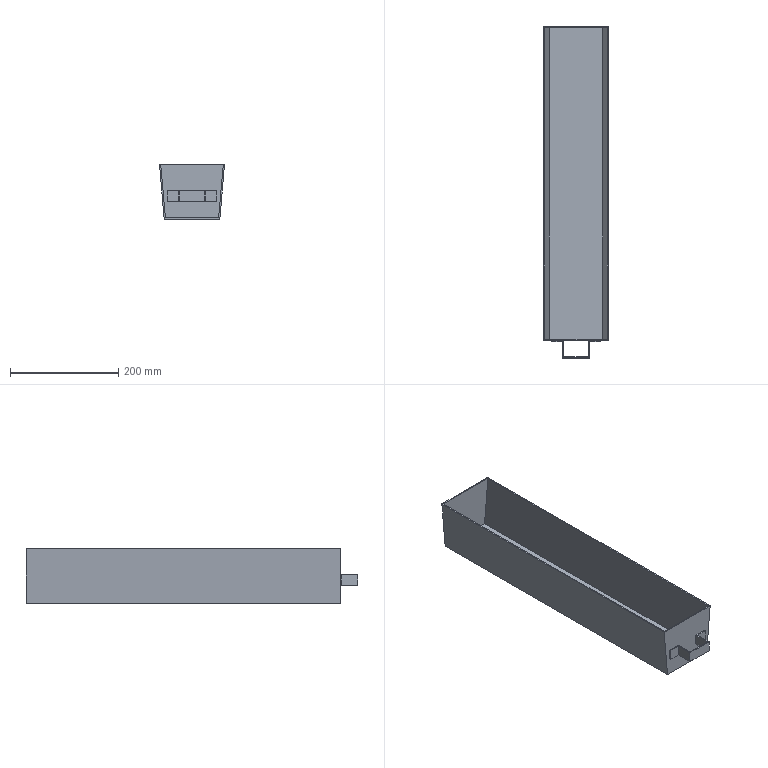Part | NX | features solid 2 | 1 solid | 23 faces | box 120 x 612.3 x 100 mm | volume 446880 mm3 | plane 19 | spline 4
STEP:
#1=CARTESIAN_POINT('',(80.865,-687.8,-515.5));
#2=VERTEX_POINT('',#1);
#3=CARTESIAN_POINT('',(179.135,-687.8,-515.5));
#4=VERTEX_POINT('',#3);
#5=CARTESIAN_POINT('',(-1370.,-687.8,-515.5));
#6=DIRECTION('',(-1.,0.,0.));
#7=VECTOR('',#6,1000.);
#8=LINE('',#5,#7);
#9=EDGE_CURVE('',#2,#4,#8,.F.);
#10=ORIENTED_EDGE('',*,*,#9,.T.);
#11=CARTESIAN_POINT('',(179.135,-112.3,-515.5));
#12=VERTEX_POINT('',#11);
#13=CARTESIAN_POINT('',(179.135,-112.3,-515.5));
#14=CARTESIAN_POINT('',(179.135,-304.133,-515.5));
#15=CARTESIAN_POINT('',(179.135,-495.967,-515.5));
#16=CARTESIAN_POINT('',(179.135,-687.8,-515.5));
#17=B_SPLINE_CURVE_WITH_KNOTS('',3,(#13,#14,#15,#16),.UNSPECIFIED.,.F.,.F.,(4,4),(0.,0.5755),.UNSPECIFIED.);
#18=EDGE_CURVE('',#12,#4,#17,.T.);
#19=ORIENTED_EDGE('',*,*,#18,.F.);
#20=CARTESIAN_POINT('',(80.865,-112.3,-515.5));
#21=VERTEX_POINT('',#20);
#22=CARTESIAN_POINT('',(896.442,-112.3,-515.5));
#23=DIRECTION('',(1.,0.,0.));
#24=VECTOR('',#23,1000.);
#25=LINE('',#22,#24);
#26=EDGE_CURVE('',#21,#12,#25,.T.);
#27=ORIENTED_EDGE('',*,*,#26,.F.);
#28=CARTESIAN_POINT('',(80.865,-687.8,-515.5));
#29=CARTESIAN_POINT('',(80.865,-495.967,-515.5));
#30=CARTESIAN_POINT('',(80.865,-304.133,-515.5));
#31=CARTESIAN_POINT('',(80.865,-112.3,-515.5));
#32=B_SPLINE_CURVE_WITH_KNOTS('',3,(#28,#29,#30,#31),.UNSPECIFIED.,.F.,.F.,(4,4),(0.,0.5755),.UNSPECIFIED.);
#33=EDGE_CURVE('',#2,#21,#32,.T.);
#34=ORIENTED_EDGE('',*,*,#33,.F.);
#35=EDGE_LOOP('',(#10,#19,#27,#34));
#36=FACE_BOUND('',#35,.T.);
#37=CARTESIAN_POINT('',(-1370.,-20.,-515.5));
#38=DIRECTION('',(0.,0.,-1.));
#39=DIRECTION('',(-1.,0.,0.));
#40=AXIS2_PLACEMENT_3D('',#37,#38,#39);
#41=PLANE('',#40);
#42=ADVANCED_FACE('',(#36),#41,.F.);
#43=CARTESIAN_POINT('',(187.691,-687.8,-417.7));
#44=VERTEX_POINT('',#43);
#45=CARTESIAN_POINT('',(187.691,-687.8,-417.7));
#46=CARTESIAN_POINT('',(184.839,-687.8,-450.3));
#47=CARTESIAN_POINT('',(181.987,-687.8,-482.9));
#48=CARTESIAN_POINT('',(179.135,-687.8,-515.5));
#49=B_SPLINE_CURVE_WITH_KNOTS('',3,(#45,#46,#47,#48),.UNSPECIFIED.,.F.,.F.,(4,4),(0.,0.09817),.UNSPECIFIED.);
#50=EDGE_CURVE('',#44,#4,#49,.T.);
#51=ORIENTED_EDGE('',*,*,#50,.F.);
#52=CARTESIAN_POINT('',(187.691,-112.3,-417.7));
#53=VERTEX_POINT('',#52);
#54=CARTESIAN_POINT('',(187.691,-112.3,-417.7));
#55=CARTESIAN_POINT('',(187.691,-304.133,-417.7));
#56=CARTESIAN_POINT('',(187.691,-495.967,-417.7));
#57=CARTESIAN_POINT('',(187.691,-687.8,-417.7));
#58=B_SPLINE_CURVE_WITH_KNOTS('',3,(#54,#55,#56,#57),.UNSPECIFIED.,.F.,.F.,(4,4),(0.,0.5755),.UNSPECIFIED.);
#59=EDGE_CURVE('',#53,#44,#58,.T.);
#60=ORIENTED_EDGE('',*,*,#59,.F.);
#61=CARTESIAN_POINT('',(187.691,-112.3,-417.7));
#62=CARTESIAN_POINT('',(184.839,-112.3,-450.3));
#63=CARTESIAN_POINT('',(181.987,-112.3,-482.9));
#64=CARTESIAN_POINT('',(179.135,-112.3,-515.5));
#65=B_SPLINE_CURVE_WITH_KNOTS('',3,(#61,#62,#63,#64),.UNSPECIFIED.,.F.,.F.,(4,4),(0.,0.09817),.UNSPECIFIED.);
#66=EDGE_CURVE('',#53,#12,#65,.T.);
#67=ORIENTED_EDGE('',*,*,#66,.T.);
#68=ORIENTED_EDGE('',*,*,#18,.T.);
#69=EDGE_LOOP('',(#51,#60,#67,#68));
#70=FACE_BOUND('',#69,.T.);
#71=CARTESIAN_POINT('',(179.135,-687.8,-515.5));
#72=CARTESIAN_POINT('',(179.135,-495.967,-515.5));
#73=CARTESIAN_POINT('',(179.135,-304.133,-515.5));
#74=CARTESIAN_POINT('',(179.135,-112.3,-515.5));
#75=CARTESIAN_POINT('',(181.987,-687.8,-482.9));
#76=CARTESIAN_POINT('',(181.987,-495.967,-482.9));
#77=CARTESIAN_POINT('',(181.987,-304.133,-482.9));
#78=CARTESIAN_POINT('',(181.987,-112.3,-482.9));
#79=CARTESIAN_POINT('',(184.839,-687.8,-450.3));
#80=CARTESIAN_POINT('',(184.839,-495.967,-450.3));
#81=CARTESIAN_POINT('',(184.839,-304.133,-450.3));
#82=CARTESIAN_POINT('',(184.839,-112.3,-450.3));
#83=CARTESIAN_POINT('',(187.691,-687.8,-417.7));
#84=CARTESIAN_POINT('',(187.691,-495.967,-417.7));
#85=CARTESIAN_POINT('',(187.691,-304.133,-417.7));
#86=CARTESIAN_POINT('',(187.691,-112.3,-417.7));
#87=B_SPLINE_SURFACE_WITH_KNOTS('',3,3,((#71,#72,#73,#74),(#75,#76,#77,#78),(#79,#80,#81,#82),(#83,#84,#85,#86)),.UNSPECIFIED.,.F.,.F.,.F.,(4,4),(4,4),(0.01625,0.998),(0.003793,0.996),.UNSPECIFIED.);
#88=ADVANCED_FACE('',(#70),#87,.T.);
#89=ORIENTED_EDGE('',*,*,#33,.T.);
#90=CARTESIAN_POINT('',(72.309,-112.3,-417.7));
#91=VERTEX_POINT('',#90);
#92=CARTESIAN_POINT('',(80.865,-112.3,-515.5));
#93=CARTESIAN_POINT('',(78.013,-112.3,-482.9));
#94=CARTESIAN_POINT('',(75.161,-112.3,-450.3));
#95=CARTESIAN_POINT('',(72.309,-112.3,-417.7));
#96=B_SPLINE_CURVE_WITH_KNOTS('',3,(#92,#93,#94,#95),.UNSPECIFIED.,.F.,.F.,(4,4),(0.,0.09817),.UNSPECIFIED.);
#97=EDGE_CURVE('',#21,#91,#96,.T.);
#98=ORIENTED_EDGE('',*,*,#97,.T.);
#99=CARTESIAN_POINT('',(72.309,-687.8,-417.7));
#100=VERTEX_POINT('',#99);
#101=CARTESIAN_POINT('',(72.309,-112.3,-417.7));
#102=CARTESIAN_POINT('',(72.309,-304.133,-417.7));
#103=CARTESIAN_POINT('',(72.309,-495.967,-417.7));
#104=CARTESIAN_POINT('',(72.309,-687.8,-417.7));
#105=B_SPLINE_CURVE_WITH_KNOTS('',3,(#101,#102,#103,#104),.UNSPECIFIED.,.F.,.F.,(4,4),(0.,0.5755),.UNSPECIFIED.);
#106=EDGE_CURVE('',#91,#100,#105,.T.);
#107=ORIENTED_EDGE('',*,*,#106,.T.);
#108=CARTESIAN_POINT('',(80.865,-687.8,-515.5));
#109=CARTESIAN_POINT('',(78.013,-687.8,-482.9));
#110=CARTESIAN_POINT('',(75.161,-687.8,-450.3));
#111=CARTESIAN_POINT('',(72.309,-687.8,-417.7));
#112=B_SPLINE_CURVE_WITH_KNOTS('',3,(#108,#109,#110,#111),.UNSPECIFIED.,.F.,.F.,(4,4),(0.,0.09817),.UNSPECIFIED.);
#113=EDGE_CURVE('',#2,#100,#112,.T.);
#114=ORIENTED_EDGE('',*,*,#113,.F.);
#115=EDGE_LOOP('',(#89,#98,#107,#114));
#116=FACE_BOUND('',#115,.T.);
#117=CARTESIAN_POINT('',(80.865,-687.8,-515.5));
#118=CARTESIAN_POINT('',(80.865,-495.967,-515.5));
#119=CARTESIAN_POINT('',(80.865,-304.133,-515.5));
#120=CARTESIAN_POINT('',(80.865,-112.3,-515.5));
#121=CARTESIAN_POINT('',(78.013,-687.8,-482.9));
#122=CARTESIAN_POINT('',(78.013,-495.967,-482.9));
#123=CARTESIAN_POINT('',(78.013,-304.133,-482.9));
#124=CARTESIAN_POINT('',(78.013,-112.3,-482.9));
#125=CARTESIAN_POINT('',(75.161,-687.8,-450.3));
#126=CARTESIAN_POINT('',(75.161,-495.967,-450.3));
#127=CARTESIAN_POINT('',(75.161,-304.133,-450.3));
#128=CARTESIAN_POINT('',(75.161,-112.3,-450.3));
#129=CARTESIAN_POINT('',(72.309,-687.8,-417.7));
#130=CARTESIAN_POINT('',(72.309,-495.967,-417.7));
#131=CARTESIAN_POINT('',(72.309,-304.133,-417.7));
#132=CARTESIAN_POINT('',(72.309,-112.3,-417.7));
#133=B_SPLINE_SURFACE_WITH_KNOTS('',3,3,((#117,#118,#119,#120),(#121,#122,#123,#124),(#125,#126,#127,#128),(#129,#130,#131,#132)),.UNSPECIFIED.,.F.,.F.,.F.,(4,4),(4,4),(0.01625,0.998),(0.003793,0.996),.UNSPECIFIED.);
#134=ADVANCED_FACE('',(#116),#133,.F.);
#135=ORIENTED_EDGE('',*,*,#59,.T.);
#136=CARTESIAN_POINT('',(-426.758,-687.8,-417.7));
#137=DIRECTION('',(1.,0.,0.));
#138=VECTOR('',#137,1000.);
#139=LINE('',#136,#138);
#140=EDGE_CURVE('',#44,#100,#139,.F.);
#141=ORIENTED_EDGE('',*,*,#140,.T.);
#142=ORIENTED_EDGE('',*,*,#106,.F.);
#143=CARTESIAN_POINT('',(896.442,-112.3,-417.7));
#144=DIRECTION('',(-1.,0.,0.));
#145=VECTOR('',#144,1000.);
#146=LINE('',#143,#145);
#147=EDGE_CURVE('',#53,#91,#146,.T.);
#148=ORIENTED_EDGE('',*,*,#147,.F.);
#149=EDGE_LOOP('',(#135,#141,#142,#148));
#150=FACE_BOUND('',#149,.T.);
#151=CARTESIAN_POINT('',(190.,-110.,-417.7));
#152=VERTEX_POINT('',#151);
#153=CARTESIAN_POINT('',(70.,-110.,-417.7));
#154=VERTEX_POINT('',#153);
#155=CARTESIAN_POINT('',(-386.442,-110.,-417.7));
#156=DIRECTION('',(-1.,0.,0.));
#157=VECTOR('',#156,1000.);
#158=LINE('',#155,#157);
#159=EDGE_CURVE('',#152,#154,#158,.T.);
#160=ORIENTED_EDGE('',*,*,#159,.T.);
#161=CARTESIAN_POINT('',(70.,-690.,-417.7));
#162=VERTEX_POINT('',#161);
#163=CARTESIAN_POINT('',(70.,-690.,-417.7));
#164=CARTESIAN_POINT('',(70.,-496.667,-417.7));
#165=CARTESIAN_POINT('',(70.,-303.333,-417.7));
#166=CARTESIAN_POINT('',(70.,-110.,-417.7));
#167=B_SPLINE_CURVE_WITH_KNOTS('',3,(#163,#164,#165,#166),.UNSPECIFIED.,.F.,.F.,(4,4),(0.,0.58),.UNSPECIFIED.);
#168=EDGE_CURVE('',#162,#154,#167,.T.);
#169=ORIENTED_EDGE('',*,*,#168,.F.);
#170=CARTESIAN_POINT('',(190.,-690.,-417.7));
#171=VERTEX_POINT('',#170);
#172=CARTESIAN_POINT('',(-426.758,-690.,-417.7));
#173=DIRECTION('',(1.,0.,0.));
#174=VECTOR('',#173,1000.);
#175=LINE('',#172,#174);
#176=EDGE_CURVE('',#171,#162,#175,.F.);
#177=ORIENTED_EDGE('',*,*,#176,.F.);
#178=CARTESIAN_POINT('',(190.,-110.,-417.7));
#179=CARTESIAN_POINT('',(190.,-303.333,-417.7));
#180=CARTESIAN_POINT('',(190.,-496.667,-417.7));
#181=CARTESIAN_POINT('',(190.,-690.,-417.7));
#182=B_SPLINE_CURVE_WITH_KNOTS('',3,(#178,#179,#180,#181),.UNSPECIFIED.,.F.,.F.,(4,4),(0.,0.58),.UNSPECIFIED.);
#183=EDGE_CURVE('',#152,#171,#182,.T.);
#184=ORIENTED_EDGE('',*,*,#183,.F.);
#185=EDGE_LOOP('',(#160,#169,#177,#184));
#186=FACE_BOUND('',#185,.T.);
#187=CARTESIAN_POINT('',(-426.758,-20.,-417.7));
#188=DIRECTION('',(0.,0.,1.));
#189=DIRECTION('',(1.,0.,0.));
#190=AXIS2_PLACEMENT_3D('',#187,#188,#189);
#191=PLANE('',#190);
#192=ADVANCED_FACE('',(#150,#186),#191,.T.);
#193=CARTESIAN_POINT('',(181.251,-110.,-517.7));
#194=VERTEX_POINT('',#193);
#195=CARTESIAN_POINT('',(181.251,-690.,-517.7));
#196=VERTEX_POINT('',#195);
#197=CARTESIAN_POINT('',(181.251,-110.,-517.7));
#198=CARTESIAN_POINT('',(181.251,-303.333,-517.7));
#199=CARTESIAN_POINT('',(181.251,-496.667,-517.7));
#200=CARTESIAN_POINT('',(181.251,-690.,-517.7));
#201=B_SPLINE_CURVE_WITH_KNOTS('',3,(#197,#198,#199,#200),.UNSPECIFIED.,.F.,.F.,(4,4),(0.,0.58),.UNSPECIFIED.);
#202=EDGE_CURVE('',#194,#196,#201,.T.);
#203=ORIENTED_EDGE('',*,*,#202,.T.);
#204=CARTESIAN_POINT('',(78.749,-690.,-517.7));
#205=VERTEX_POINT('',#204);
#206=CARTESIAN_POINT('',(-1370.,-690.,-517.7));
#207=DIRECTION('',(1.,0.,0.));
#208=VECTOR('',#207,1000.);
#209=LINE('',#206,#208);
#210=EDGE_CURVE('',#205,#196,#209,.T.);
#211=ORIENTED_EDGE('',*,*,#210,.F.);
#212=CARTESIAN_POINT('',(78.749,-110.,-517.7));
#213=VERTEX_POINT('',#212);
#214=CARTESIAN_POINT('',(78.749,-110.,-517.7));
#215=CARTESIAN_POINT('',(78.749,-303.333,-517.7));
#216=CARTESIAN_POINT('',(78.749,-496.667,-517.7));
#217=CARTESIAN_POINT('',(78.749,-690.,-517.7));
#218=B_SPLINE_CURVE_WITH_KNOTS('',3,(#214,#215,#216,#217),.UNSPECIFIED.,.F.,.F.,(4,4),(0.,0.58),.UNSPECIFIED.);
#219=EDGE_CURVE('',#213,#205,#218,.T.);
#220=ORIENTED_EDGE('',*,*,#219,.F.);
#221=CARTESIAN_POINT('',(-386.442,-110.,-517.7));
#222=DIRECTION('',(1.,0.,0.));
#223=VECTOR('',#222,1000.);
#224=LINE('',#221,#223);
#225=EDGE_CURVE('',#213,#194,#224,.T.);
#226=ORIENTED_EDGE('',*,*,#225,.T.);
#227=EDGE_LOOP('',(#203,#211,#220,#226));
#228=FACE_BOUND('',#227,.T.);
#229=CARTESIAN_POINT('',(-1370.,-20.,-517.7));
#230=DIRECTION('',(0.,0.,-1.));
#231=DIRECTION('',(-1.,0.,0.));
#232=AXIS2_PLACEMENT_3D('',#229,#230,#231);
#233=PLANE('',#232);
#234=ADVANCED_FACE('',(#228),#233,.T.);
#235=ORIENTED_EDGE('',*,*,#183,.T.);
#236=CARTESIAN_POINT('',(190.,-690.,-417.7));
#237=CARTESIAN_POINT('',(187.084,-690.,-451.033));
#238=CARTESIAN_POINT('',(184.167,-690.,-484.367));
#239=CARTESIAN_POINT('',(181.251,-690.,-517.7));
#240=B_SPLINE_CURVE_WITH_KNOTS('',3,(#236,#237,#238,#239),.UNSPECIFIED.,.F.,.F.,(4,4),(0.,0.1004),.UNSPECIFIED.);
#241=EDGE_CURVE('',#171,#196,#240,.T.);
#242=ORIENTED_EDGE('',*,*,#241,.T.);
#243=ORIENTED_EDGE('',*,*,#202,.F.);
#244=CARTESIAN_POINT('',(190.,-110.,-417.7));
#245=CARTESIAN_POINT('',(187.084,-110.,-451.033));
#246=CARTESIAN_POINT('',(184.167,-110.,-484.367));
#247=CARTESIAN_POINT('',(181.251,-110.,-517.7));
#248=B_SPLINE_CURVE_WITH_KNOTS('',3,(#244,#245,#246,#247),.UNSPECIFIED.,.F.,.F.,(4,4),(0.,0.1004),.UNSPECIFIED.);
#249=EDGE_CURVE('',#152,#194,#248,.T.);
#250=ORIENTED_EDGE('',*,*,#249,.F.);
#251=EDGE_LOOP('',(#235,#242,#243,#250));
#252=FACE_BOUND('',#251,.T.);
#253=CARTESIAN_POINT('',(181.197,-690.,-518.316));
#254=CARTESIAN_POINT('',(181.197,-110.,-518.316));
#255=CARTESIAN_POINT('',(181.284,-690.,-517.319));
#256=CARTESIAN_POINT('',(181.284,-110.,-517.319));
#257=CARTESIAN_POINT('',(190.,-690.,-417.7));
#258=CARTESIAN_POINT('',(190.,-110.,-417.7));
#259=B_SPLINE_SURFACE_WITH_KNOTS('',1,1,((#253,#254),(#255,#256),(#257,#258)),.PLANE_SURF.,.F.,.F.,.F.,(2,1,2),(2,2),(-0.01,0.,1.),(0.,1.),.PIECEWISE_BEZIER_KNOTS.);
#260=ADVANCED_FACE('',(#252),#259,.F.);
#261=ORIENTED_EDGE('',*,*,#219,.T.);
#262=CARTESIAN_POINT('',(70.,-690.,-417.7));
#263=CARTESIAN_POINT('',(72.916,-690.,-451.033));
#264=CARTESIAN_POINT('',(75.833,-690.,-484.367));
#265=CARTESIAN_POINT('',(78.749,-690.,-517.7));
#266=B_SPLINE_CURVE_WITH_KNOTS('',3,(#262,#263,#264,#265),.UNSPECIFIED.,.F.,.F.,(4,4),(0.,0.1004),.UNSPECIFIED.);
#267=EDGE_CURVE('',#162,#205,#266,.T.);
#268=ORIENTED_EDGE('',*,*,#267,.F.);
#269=ORIENTED_EDGE('',*,*,#168,.T.);
#270=CARTESIAN_POINT('',(78.749,-110.,-517.7));
#271=CARTESIAN_POINT('',(75.833,-110.,-484.367));
#272=CARTESIAN_POINT('',(72.916,-110.,-451.033));
#273=CARTESIAN_POINT('',(70.,-110.,-417.7));
#274=B_SPLINE_CURVE_WITH_KNOTS('',3,(#270,#271,#272,#273),.UNSPECIFIED.,.F.,.F.,(4,4),(0.,0.1004),.UNSPECIFIED.);
#275=EDGE_CURVE('',#213,#154,#274,.T.);
#276=ORIENTED_EDGE('',*,*,#275,.F.);
#277=EDGE_LOOP('',(#261,#268,#269,#276));
#278=FACE_BOUND('',#277,.T.);
#279=CARTESIAN_POINT('',(78.803,-690.,-518.316));
#280=CARTESIAN_POINT('',(78.803,-110.,-518.316));
#281=CARTESIAN_POINT('',(78.716,-690.,-517.319));
#282=CARTESIAN_POINT('',(78.716,-110.,-517.319));
#283=CARTESIAN_POINT('',(70.,-690.,-417.7));
#284=CARTESIAN_POINT('',(70.,-110.,-417.7));
#285=B_SPLINE_SURFACE_WITH_KNOTS('',1,1,((#279,#280),(#281,#282),(#283,#284)),.PLANE_SURF.,.F.,.F.,.F.,(2,1,2),(2,2),(-0.01,0.,1.),(0.,1.),.PIECEWISE_BEZIER_KNOTS.);
#286=ADVANCED_FACE('',(#278),#285,.T.);
#287=CARTESIAN_POINT('',(85.,-690.,-465.2));
#288=VERTEX_POINT('',#287);
#289=CARTESIAN_POINT('',(107.3,-690.,-465.2));
#290=VERTEX_POINT('',#289);
#291=CARTESIAN_POINT('',(105.,-690.,-465.2));
#292=DIRECTION('',(-1.,0.,0.));
#293=VECTOR('',#292,1000.);
#294=LINE('',#291,#293);
#295=EDGE_CURVE('',#288,#290,#294,.F.);
#296=ORIENTED_EDGE('',*,*,#295,.T.);
#297=CARTESIAN_POINT('',(107.3,-690.,-485.2));
#298=VERTEX_POINT('',#297);
#299=CARTESIAN_POINT('',(107.3,-690.,-485.2));
#300=DIRECTION('',(0.,0.,1.));
#301=VECTOR('',#300,1000.);
#302=LINE('',#299,#301);
#303=EDGE_CURVE('',#298,#290,#302,.T.);
#304=ORIENTED_EDGE('',*,*,#303,.F.);
#305=CARTESIAN_POINT('',(85.,-690.,-485.2));
#306=VERTEX_POINT('',#305);
#307=CARTESIAN_POINT('',(105.,-690.,-485.2));
#308=DIRECTION('',(-1.,0.,0.));
#309=VECTOR('',#308,1000.);
#310=LINE('',#307,#309);
#311=EDGE_CURVE('',#298,#306,#310,.T.);
#312=ORIENTED_EDGE('',*,*,#311,.T.);
#313=CARTESIAN_POINT('',(85.,-690.,-485.2));
#314=DIRECTION('',(0.,0.,1.));
#315=VECTOR('',#314,1000.);
#316=LINE('',#313,#315);
#317=EDGE_CURVE('',#306,#288,#316,.T.);
#318=ORIENTED_EDGE('',*,*,#317,.T.);
#319=EDGE_LOOP('',(#296,#304,#312,#318));
#320=FACE_BOUND('',#319,.T.);
#321=ORIENTED_EDGE('',*,*,#210,.T.);
#322=ORIENTED_EDGE('',*,*,#241,.F.);
#323=ORIENTED_EDGE('',*,*,#176,.T.);
#324=ORIENTED_EDGE('',*,*,#267,.T.);
#325=EDGE_LOOP('',(#321,#322,#323,#324));
#326=FACE_BOUND('',#325,.T.);
#327=CARTESIAN_POINT('',(152.7,-690.,-465.2));
#328=VERTEX_POINT('',#327);
#329=CARTESIAN_POINT('',(175.,-690.,-465.2));
#330=VERTEX_POINT('',#329);
#331=CARTESIAN_POINT('',(105.,-690.,-465.2));
#332=DIRECTION('',(-1.,0.,0.));
#333=VECTOR('',#332,1000.);
#334=LINE('',#331,#333);
#335=EDGE_CURVE('',#328,#330,#334,.F.);
#336=ORIENTED_EDGE('',*,*,#335,.T.);
#337=CARTESIAN_POINT('',(175.,-690.,-485.2));
#338=VERTEX_POINT('',#337);
#339=CARTESIAN_POINT('',(175.,-690.,-485.2));
#340=DIRECTION('',(0.,0.,1.));
#341=VECTOR('',#340,1000.);
#342=LINE('',#339,#341);
#343=EDGE_CURVE('',#338,#330,#342,.T.);
#344=ORIENTED_EDGE('',*,*,#343,.F.);
#345=CARTESIAN_POINT('',(152.7,-690.,-485.2));
#346=VERTEX_POINT('',#345);
#347=CARTESIAN_POINT('',(105.,-690.,-485.2));
#348=DIRECTION('',(-1.,0.,0.));
#349=VECTOR('',#348,1000.);
#350=LINE('',#347,#349);
#351=EDGE_CURVE('',#338,#346,#350,.T.);
#352=ORIENTED_EDGE('',*,*,#351,.T.);
#353=CARTESIAN_POINT('',(152.7,-690.,-485.2));
#354=DIRECTION('',(0.,0.,-1.));
#355=VECTOR('',#354,1000.);
#356=LINE('',#353,#355);
#357=EDGE_CURVE('',#346,#328,#356,.F.);
#358=ORIENTED_EDGE('',*,*,#357,.T.);
#359=EDGE_LOOP('',(#336,#344,#352,#358));
#360=FACE_BOUND('',#359,.T.);
#361=CARTESIAN_POINT('',(280.,-690.,-137.7));
#362=DIRECTION('',(0.,-1.,0.));
#363=DIRECTION('',(0.,0.,-1.));
#364=AXIS2_PLACEMENT_3D('',#361,#362,#363);
#365=PLANE('',#364);
#366=ADVANCED_FACE('',(#320,#326,#360),#365,.T.);
#367=ORIENTED_EDGE('',*,*,#9,.F.);
#368=ORIENTED_EDGE('',*,*,#113,.T.);
#369=ORIENTED_EDGE('',*,*,#140,.F.);
#370=ORIENTED_EDGE('',*,*,#50,.T.);
#371=EDGE_LOOP('',(#367,#368,#369,#370));
#372=FACE_BOUND('',#371,.T.);
#373=CARTESIAN_POINT('',(280.,-687.8,-137.7));
#374=DIRECTION('',(0.,-1.,0.));
#375=DIRECTION('',(0.,0.,-1.));
#376=AXIS2_PLACEMENT_3D('',#373,#374,#375);
#377=PLANE('',#376);
#378=ADVANCED_FACE('',(#372),#377,.F.);
#379=CARTESIAN_POINT('',(105.,-692.3,-485.2));
#380=VERTEX_POINT('',#379);
#381=CARTESIAN_POINT('',(105.,-692.3,-465.2));
#382=VERTEX_POINT('',#381);
#383=CARTESIAN_POINT('',(105.,-692.3,-485.2));
#384=DIRECTION('',(0.,0.,-1.));
#385=VECTOR('',#384,1000.);
#386=LINE('',#383,#385);
#387=EDGE_CURVE('',#380,#382,#386,.F.);
#388=ORIENTED_EDGE('',*,*,#387,.F.);
#389=CARTESIAN_POINT('',(105.,-722.3,-485.2));
#390=VERTEX_POINT('',#389);
#391=CARTESIAN_POINT('',(105.,-732.3,-485.2));
#392=DIRECTION('',(0.,1.,0.));
#393=VECTOR('',#392,1000.);
#394=LINE('',#391,#393);
#395=EDGE_CURVE('',#390,#380,#394,.T.);
#396=ORIENTED_EDGE('',*,*,#395,.F.);
#397=CARTESIAN_POINT('',(105.,-722.3,-465.2));
#398=VERTEX_POINT('',#397);
#399=CARTESIAN_POINT('',(105.,-722.3,-485.2));
#400=DIRECTION('',(0.,0.,1.));
#401=VECTOR('',#400,1000.);
#402=LINE('',#399,#401);
#403=EDGE_CURVE('',#390,#398,#402,.T.);
#404=ORIENTED_EDGE('',*,*,#403,.T.);
#405=CARTESIAN_POINT('',(105.,-732.3,-465.2));
#406=DIRECTION('',(0.,1.,0.));
#407=VECTOR('',#406,1000.);
#408=LINE('',#405,#407);
#409=EDGE_CURVE('',#398,#382,#408,.T.);
#410=ORIENTED_EDGE('',*,*,#409,.T.);
#411=EDGE_LOOP('',(#388,#396,#404,#410));
#412=FACE_BOUND('',#411,.T.);
#413=CARTESIAN_POINT('',(105.,-732.3,-485.2));
#414=DIRECTION('',(-1.,0.,0.));
#415=DIRECTION('',(0.,0.,1.));
#416=AXIS2_PLACEMENT_3D('',#413,#414,#415);
#417=PLANE('',#416);
#418=ADVANCED_FACE('',(#412),#417,.T.);
#419=CARTESIAN_POINT('',(85.,-692.3,-485.2));
#420=VERTEX_POINT('',#419);
#421=CARTESIAN_POINT('',(85.,-692.3,-465.2));
#422=VERTEX_POINT('',#421);
#423=CARTESIAN_POINT('',(85.,-692.3,-485.2));
#424=DIRECTION('',(0.,0.,-1.));
#425=VECTOR('',#424,1000.);
#426=LINE('',#423,#425);
#427=EDGE_CURVE('',#420,#422,#426,.F.);
#428=ORIENTED_EDGE('',*,*,#427,.F.);
#429=CARTESIAN_POINT('',(105.,-692.3,-485.2));
#430=DIRECTION('',(1.,0.,0.));
#431=VECTOR('',#430,1000.);
#432=LINE('',#429,#431);
#433=EDGE_CURVE('',#380,#420,#432,.F.);
#434=ORIENTED_EDGE('',*,*,#433,.F.);
#435=ORIENTED_EDGE('',*,*,#387,.T.);
#436=CARTESIAN_POINT('',(105.,-692.3,-465.2));
#437=DIRECTION('',(1.,0.,0.));
#438=VECTOR('',#437,1000.);
#439=LINE('',#436,#438);
#440=EDGE_CURVE('',#382,#422,#439,.F.);
#441=ORIENTED_EDGE('',*,*,#440,.T.);
#442=EDGE_LOOP('',(#428,#434,#435,#441));
#443=FACE_BOUND('',#442,.T.);
#444=CARTESIAN_POINT('',(105.,-692.3,-485.2));
#445=DIRECTION('',(0.,-1.,0.));
#446=DIRECTION('',(0.,0.,-1.));
#447=AXIS2_PLACEMENT_3D('',#444,#445,#446);
#448=PLANE('',#447);
#449=ADVANCED_FACE('',(#443),#448,.T.);
#450=CARTESIAN_POINT('',(155.,-692.3,-485.2));
#451=VERTEX_POINT('',#450);
#452=CARTESIAN_POINT('',(155.,-722.3,-485.2));
#453=VERTEX_POINT('',#452);
#454=CARTESIAN_POINT('',(155.,-720.,-485.2));
#455=DIRECTION('',(0.,1.,0.));
#456=VECTOR('',#455,1000.);
#457=LINE('',#454,#456);
#458=EDGE_CURVE('',#451,#453,#457,.F.);
#459=ORIENTED_EDGE('',*,*,#458,.F.);
#460=CARTESIAN_POINT('',(155.,-692.3,-465.2));
#461=VERTEX_POINT('',#460);
#462=CARTESIAN_POINT('',(155.,-692.3,-485.2));
#463=DIRECTION('',(0.,0.,1.));
#464=VECTOR('',#463,1000.);
#465=LINE('',#462,#464);
#466=EDGE_CURVE('',#451,#461,#465,.T.);
#467=ORIENTED_EDGE('',*,*,#466,.T.);
#468=CARTESIAN_POINT('',(155.,-722.3,-465.2));
#469=VERTEX_POINT('',#468);
#470=CARTESIAN_POINT('',(155.,-720.,-465.2));
#471=DIRECTION('',(0.,-1.,0.));
#472=VECTOR('',#471,1000.);
#473=LINE('',#470,#472);
#474=EDGE_CURVE('',#461,#469,#473,.T.);
#475=ORIENTED_EDGE('',*,*,#474,.T.);
#476=CARTESIAN_POINT('',(155.,-722.3,-485.2));
#477=DIRECTION('',(0.,0.,1.));
#478=VECTOR('',#477,1000.);
#479=LINE('',#476,#478);
#480=EDGE_CURVE('',#453,#469,#479,.T.);
#481=ORIENTED_EDGE('',*,*,#480,.F.);
#482=EDGE_LOOP('',(#459,#467,#475,#481));
#483=FACE_BOUND('',#482,.T.);
#484=CARTESIAN_POINT('',(155.,-720.,-485.2));
#485=DIRECTION('',(-1.,0.,0.));
#486=DIRECTION('',(0.,0.,1.));
#487=AXIS2_PLACEMENT_3D('',#484,#485,#486);
#488=PLANE('',#487);
#489=ADVANCED_FACE('',(#483),#488,.F.);
#490=CARTESIAN_POINT('',(105.,-722.3,-485.2));
#491=DIRECTION('',(-1.,0.,0.));
#492=VECTOR('',#491,1000.);
#493=LINE('',#490,#492);
#494=EDGE_CURVE('',#390,#453,#493,.F.);
#495=ORIENTED_EDGE('',*,*,#494,.T.);
#496=ORIENTED_EDGE('',*,*,#480,.T.);
#497=CARTESIAN_POINT('',(277.5,-722.3,-465.2));
#498=DIRECTION('',(1.,0.,0.));
#499=VECTOR('',#498,1000.);
#500=LINE('',#497,#499);
#501=EDGE_CURVE('',#398,#469,#500,.T.);
#502=ORIENTED_EDGE('',*,*,#501,.F.);
#503=ORIENTED_EDGE('',*,*,#403,.F.);
#504=EDGE_LOOP('',(#495,#496,#502,#503));
#505=FACE_BOUND('',#504,.T.);
#506=CARTESIAN_POINT('',(277.5,-722.3,-485.2));
#507=DIRECTION('',(0.,1.,0.));
#508=DIRECTION('',(0.,0.,1.));
#509=AXIS2_PLACEMENT_3D('',#506,#507,#508);
#510=PLANE('',#509);
#511=ADVANCED_FACE('',(#505),#510,.F.);
#512=CARTESIAN_POINT('',(152.7,-720.,-485.2));
#513=VERTEX_POINT('',#512);
#514=CARTESIAN_POINT('',(152.7,-720.,-465.2));
#515=VERTEX_POINT('',#514);
#516=CARTESIAN_POINT('',(152.7,-720.,-485.2));
#517=DIRECTION('',(0.,0.,-1.));
#518=VECTOR('',#517,1000.);
#519=LINE('',#516,#518);
#520=EDGE_CURVE('',#513,#515,#519,.F.);
#521=ORIENTED_EDGE('',*,*,#520,.F.);
#522=CARTESIAN_POINT('',(107.3,-720.,-485.2));
#523=VERTEX_POINT('',#522);
#524=CARTESIAN_POINT('',(277.5,-720.,-485.2));
#525=DIRECTION('',(-1.,0.,0.));
#526=VECTOR('',#525,1000.);
#527=LINE('',#524,#526);
#528=EDGE_CURVE('',#513,#523,#527,.T.);
#529=ORIENTED_EDGE('',*,*,#528,.T.);
#530=CARTESIAN_POINT('',(107.3,-720.,-465.2));
#531=VERTEX_POINT('',#530);
#532=CARTESIAN_POINT('',(107.3,-720.,-485.2));
#533=DIRECTION('',(0.,0.,-1.));
#534=VECTOR('',#533,1000.);
#535=LINE('',#532,#534);
#536=EDGE_CURVE('',#523,#531,#535,.F.);
#537=ORIENTED_EDGE('',*,*,#536,.T.);
#538=CARTESIAN_POINT('',(277.5,-720.,-465.2));
#539=DIRECTION('',(-1.,0.,0.));
#540=VECTOR('',#539,1000.);
#541=LINE('',#538,#540);
#542=EDGE_CURVE('',#515,#531,#541,.T.);
#543=ORIENTED_EDGE('',*,*,#542,.F.);
#544=EDGE_LOOP('',(#521,#529,#537,#543));
#545=FACE_BOUND('',#544,.T.);
#546=CARTESIAN_POINT('',(277.5,-720.,-485.2));
#547=DIRECTION('',(0.,1.,0.));
#548=DIRECTION('',(0.,0.,1.));
#549=AXIS2_PLACEMENT_3D('',#546,#547,#548);
#550=PLANE('',#549);
#551=ADVANCED_FACE('',(#545),#550,.T.);
#552=CARTESIAN_POINT('',(175.,-692.3,-485.2));
#553=VERTEX_POINT('',#552);
#554=CARTESIAN_POINT('',(175.,-692.3,-465.2));
#555=VERTEX_POINT('',#554);
#556=CARTESIAN_POINT('',(175.,-692.3,-485.2));
#557=DIRECTION('',(0.,0.,1.));
#558=VECTOR('',#557,1000.);
#559=LINE('',#556,#558);
#560=EDGE_CURVE('',#553,#555,#559,.T.);
#561=ORIENTED_EDGE('',*,*,#560,.T.);
#562=CARTESIAN_POINT('',(155.,-692.3,-465.2));
#563=DIRECTION('',(1.,0.,0.));
#564=VECTOR('',#563,1000.);
#565=LINE('',#562,#564);
#566=EDGE_CURVE('',#461,#555,#565,.T.);
#567=ORIENTED_EDGE('',*,*,#566,.F.);
#568=ORIENTED_EDGE('',*,*,#466,.F.);
#569=CARTESIAN_POINT('',(155.,-692.3,-485.2));
#570=DIRECTION('',(1.,0.,0.));
#571=VECTOR('',#570,1000.);
#572=LINE('',#569,#571);
#573=EDGE_CURVE('',#451,#553,#572,.T.);
#574=ORIENTED_EDGE('',*,*,#573,.T.);
#575=EDGE_LOOP('',(#561,#567,#568,#574));
#576=FACE_BOUND('',#575,.T.);
#577=CARTESIAN_POINT('',(155.,-692.3,-485.2));
#578=DIRECTION('',(0.,1.,0.));
#579=DIRECTION('',(0.,0.,1.));
#580=AXIS2_PLACEMENT_3D('',#577,#578,#579);
#581=PLANE('',#580);
#582=ADVANCED_FACE('',(#576),#581,.F.);
#583=ORIENTED_EDGE('',*,*,#536,.F.);
#584=CARTESIAN_POINT('',(107.3,-732.3,-485.2));
#585=DIRECTION('',(0.,1.,0.));
#586=VECTOR('',#585,1000.);
#587=LINE('',#584,#586);
#588=EDGE_CURVE('',#523,#298,#587,.T.);
#589=ORIENTED_EDGE('',*,*,#588,.T.);
#590=ORIENTED_EDGE('',*,*,#303,.T.);
#591=CARTESIAN_POINT('',(107.3,-732.3,-465.2));
#592=DIRECTION('',(0.,1.,0.));
#593=VECTOR('',#592,1000.);
#594=LINE('',#591,#593);
#595=EDGE_CURVE('',#531,#290,#594,.T.);
#596=ORIENTED_EDGE('',*,*,#595,.F.);
#597=EDGE_LOOP('',(#583,#589,#590,#596));
#598=FACE_BOUND('',#597,.T.);
#599=CARTESIAN_POINT('',(107.3,-732.3,-485.2));
#600=DIRECTION('',(-1.,0.,0.));
#601=DIRECTION('',(0.,0.,1.));
#602=AXIS2_PLACEMENT_3D('',#599,#600,#601);
#603=PLANE('',#602);
#604=ADVANCED_FACE('',(#598),#603,.F.);
#605=CARTESIAN_POINT('',(152.7,-732.3,-485.2));
#606=DIRECTION('',(0.,1.,0.));
#607=VECTOR('',#606,1000.);
#608=LINE('',#605,#607);
#609=EDGE_CURVE('',#513,#346,#608,.T.);
#610=ORIENTED_EDGE('',*,*,#609,.F.);
#611=ORIENTED_EDGE('',*,*,#520,.T.);
#612=CARTESIAN_POINT('',(152.7,-732.3,-465.2));
#613=DIRECTION('',(0.,1.,0.));
#614=VECTOR('',#613,1000.);
#615=LINE('',#612,#614);
#616=EDGE_CURVE('',#515,#328,#615,.T.);
#617=ORIENTED_EDGE('',*,*,#616,.T.);
#618=ORIENTED_EDGE('',*,*,#357,.F.);
#619=EDGE_LOOP('',(#610,#611,#617,#618));
#620=FACE_BOUND('',#619,.T.);
#621=CARTESIAN_POINT('',(152.7,-732.3,-485.2));
#622=DIRECTION('',(1.,0.,0.));
#623=DIRECTION('',(0.,0.,1.));
#624=AXIS2_PLACEMENT_3D('',#621,#622,#623);
#625=PLANE('',#624);
#626=ADVANCED_FACE('',(#620),#625,.F.);
#627=CARTESIAN_POINT('',(175.,-690.,-465.2));
#628=DIRECTION('',(0.,1.,0.));
#629=VECTOR('',#628,1000.);
#630=LINE('',#627,#629);
#631=EDGE_CURVE('',#330,#555,#630,.F.);
#632=ORIENTED_EDGE('',*,*,#631,.T.);
#633=ORIENTED_EDGE('',*,*,#560,.F.);
#634=CARTESIAN_POINT('',(175.,-690.,-485.2));
#635=DIRECTION('',(0.,1.,0.));
#636=VECTOR('',#635,1000.);
#637=LINE('',#634,#636);
#638=EDGE_CURVE('',#338,#553,#637,.F.);
#639=ORIENTED_EDGE('',*,*,#638,.F.);
#640=ORIENTED_EDGE('',*,*,#343,.T.);
#641=EDGE_LOOP('',(#632,#633,#639,#640));
#642=FACE_BOUND('',#641,.T.);
#643=CARTESIAN_POINT('',(175.,-690.,-485.2));
#644=DIRECTION('',(-1.,0.,0.));
#645=DIRECTION('',(0.,0.,1.));
#646=AXIS2_PLACEMENT_3D('',#643,#644,#645);
#647=PLANE('',#646);
#648=ADVANCED_FACE('',(#642),#647,.F.);
#649=ORIENTED_EDGE('',*,*,#501,.T.);
#650=ORIENTED_EDGE('',*,*,#474,.F.);
#651=ORIENTED_EDGE('',*,*,#566,.T.);
#652=ORIENTED_EDGE('',*,*,#631,.F.);
#653=ORIENTED_EDGE('',*,*,#335,.F.);
#654=ORIENTED_EDGE('',*,*,#616,.F.);
#655=ORIENTED_EDGE('',*,*,#542,.T.);
#656=ORIENTED_EDGE('',*,*,#595,.T.);
#657=ORIENTED_EDGE('',*,*,#295,.F.);
#658=CARTESIAN_POINT('',(85.,-690.,-465.2));
#659=DIRECTION('',(0.,1.,0.));
#660=VECTOR('',#659,1000.);
#661=LINE('',#658,#660);
#662=EDGE_CURVE('',#288,#422,#661,.F.);
#663=ORIENTED_EDGE('',*,*,#662,.T.);
#664=ORIENTED_EDGE('',*,*,#440,.F.);
#665=ORIENTED_EDGE('',*,*,#409,.F.);
#666=EDGE_LOOP('',(#649,#650,#651,#652,#653,#654,#655,#656,#657,#663,#664,#665));
#667=FACE_BOUND('',#666,.T.);
#668=CARTESIAN_POINT('',(105.,-690.,-465.2));
#669=DIRECTION('',(0.,0.,1.));
#670=DIRECTION('',(-1.,0.,0.));
#671=AXIS2_PLACEMENT_3D('',#668,#669,#670);
#672=PLANE('',#671);
#673=ADVANCED_FACE('',(#667),#672,.T.);
#674=CARTESIAN_POINT('',(85.,-690.,-485.2));
#675=DIRECTION('',(0.,1.,0.));
#676=VECTOR('',#675,1000.);
#677=LINE('',#674,#676);
#678=EDGE_CURVE('',#306,#420,#677,.F.);
#679=ORIENTED_EDGE('',*,*,#678,.T.);
#680=ORIENTED_EDGE('',*,*,#427,.T.);
#681=ORIENTED_EDGE('',*,*,#662,.F.);
#682=ORIENTED_EDGE('',*,*,#317,.F.);
#683=EDGE_LOOP('',(#679,#680,#681,#682));
#684=FACE_BOUND('',#683,.T.);
#685=CARTESIAN_POINT('',(85.,-690.,-485.2));
#686=DIRECTION('',(1.,0.,0.));
#687=DIRECTION('',(0.,0.,1.));
#688=AXIS2_PLACEMENT_3D('',#685,#686,#687);
#689=PLANE('',#688);
#690=ADVANCED_FACE('',(#684),#689,.F.);
#691=ORIENTED_EDGE('',*,*,#528,.F.);
#692=ORIENTED_EDGE('',*,*,#609,.T.);
#693=ORIENTED_EDGE('',*,*,#351,.F.);
#694=ORIENTED_EDGE('',*,*,#638,.T.);
#695=ORIENTED_EDGE('',*,*,#573,.F.);
#696=ORIENTED_EDGE('',*,*,#458,.T.);
#697=ORIENTED_EDGE('',*,*,#494,.F.);
#698=ORIENTED_EDGE('',*,*,#395,.T.);
#699=ORIENTED_EDGE('',*,*,#433,.T.);
#700=ORIENTED_EDGE('',*,*,#678,.F.);
#701=ORIENTED_EDGE('',*,*,#311,.F.);
#702=ORIENTED_EDGE('',*,*,#588,.F.);
#703=EDGE_LOOP('',(#691,#692,#693,#694,#695,#696,#697,#698,#699,#700,#701,#702));
#704=FACE_BOUND('',#703,.T.);
#705=CARTESIAN_POINT('',(105.,-690.,-485.2));
#706=DIRECTION('',(0.,0.,1.));
#707=DIRECTION('',(-1.,0.,0.));
#708=AXIS2_PLACEMENT_3D('',#705,#706,#707);
#709=PLANE('',#708);
#710=ADVANCED_FACE('',(#704),#709,.F.);
#711=ORIENTED_EDGE('',*,*,#159,.F.);
#712=ORIENTED_EDGE('',*,*,#249,.T.);
#713=ORIENTED_EDGE('',*,*,#225,.F.);
#714=ORIENTED_EDGE('',*,*,#275,.T.);
#715=EDGE_LOOP('',(#711,#712,#713,#714));
#716=FACE_BOUND('',#715,.T.);
#717=CARTESIAN_POINT('',(-386.442,-110.,-247.7));
#718=DIRECTION('',(0.,1.,0.));
#719=DIRECTION('',(0.,0.,1.));
#720=AXIS2_PLACEMENT_3D('',#717,#718,#719);
#721=PLANE('',#720);
#722=ADVANCED_FACE('',(#716),#721,.T.);
#723=ORIENTED_EDGE('',*,*,#97,.F.);
#724=ORIENTED_EDGE('',*,*,#26,.T.);
#725=ORIENTED_EDGE('',*,*,#66,.F.);
#726=ORIENTED_EDGE('',*,*,#147,.T.);
#727=EDGE_LOOP('',(#723,#724,#725,#726));
#728=FACE_BOUND('',#727,.T.);
#729=CARTESIAN_POINT('',(896.442,-112.3,-167.7));
#730=DIRECTION('',(0.,1.,0.));
#731=DIRECTION('',(0.,0.,1.));
#732=AXIS2_PLACEMENT_3D('',#729,#730,#731);
#733=PLANE('',#732);
#734=ADVANCED_FACE('',(#728),#733,.F.);
#735=CLOSED_SHELL('',(#42,#88,#134,#192,#234,#260,#286,#366,#378,#418,#449,#489,#511,#551,#582,#604,#626,#648,#673,#690,#710,#722,#734));
#736=MANIFOLD_SOLID_BREP('',#735);
#737=(LENGTH_UNIT()NAMED_UNIT(*)SI_UNIT(.MILLI.,.METRE.));
#738=UNCERTAINTY_MEASURE_WITH_UNIT(LENGTH_MEASURE(0.0508),#737,'','');
#739=(NAMED_UNIT(*)PLANE_ANGLE_UNIT()SI_UNIT($,.RADIAN.));
#740=(NAMED_UNIT(*)SI_UNIT($,.STERADIAN.)SOLID_ANGLE_UNIT());
#741=(GEOMETRIC_REPRESENTATION_CONTEXT(3)GLOBAL_UNCERTAINTY_ASSIGNED_CONTEXT((#738))GLOBAL_UNIT_ASSIGNED_CONTEXT((#737,#739,#740))REPRESENTATION_CONTEXT('',''));
#742=ADVANCED_BREP_SHAPE_REPRESENTATION('',(#736),#741);